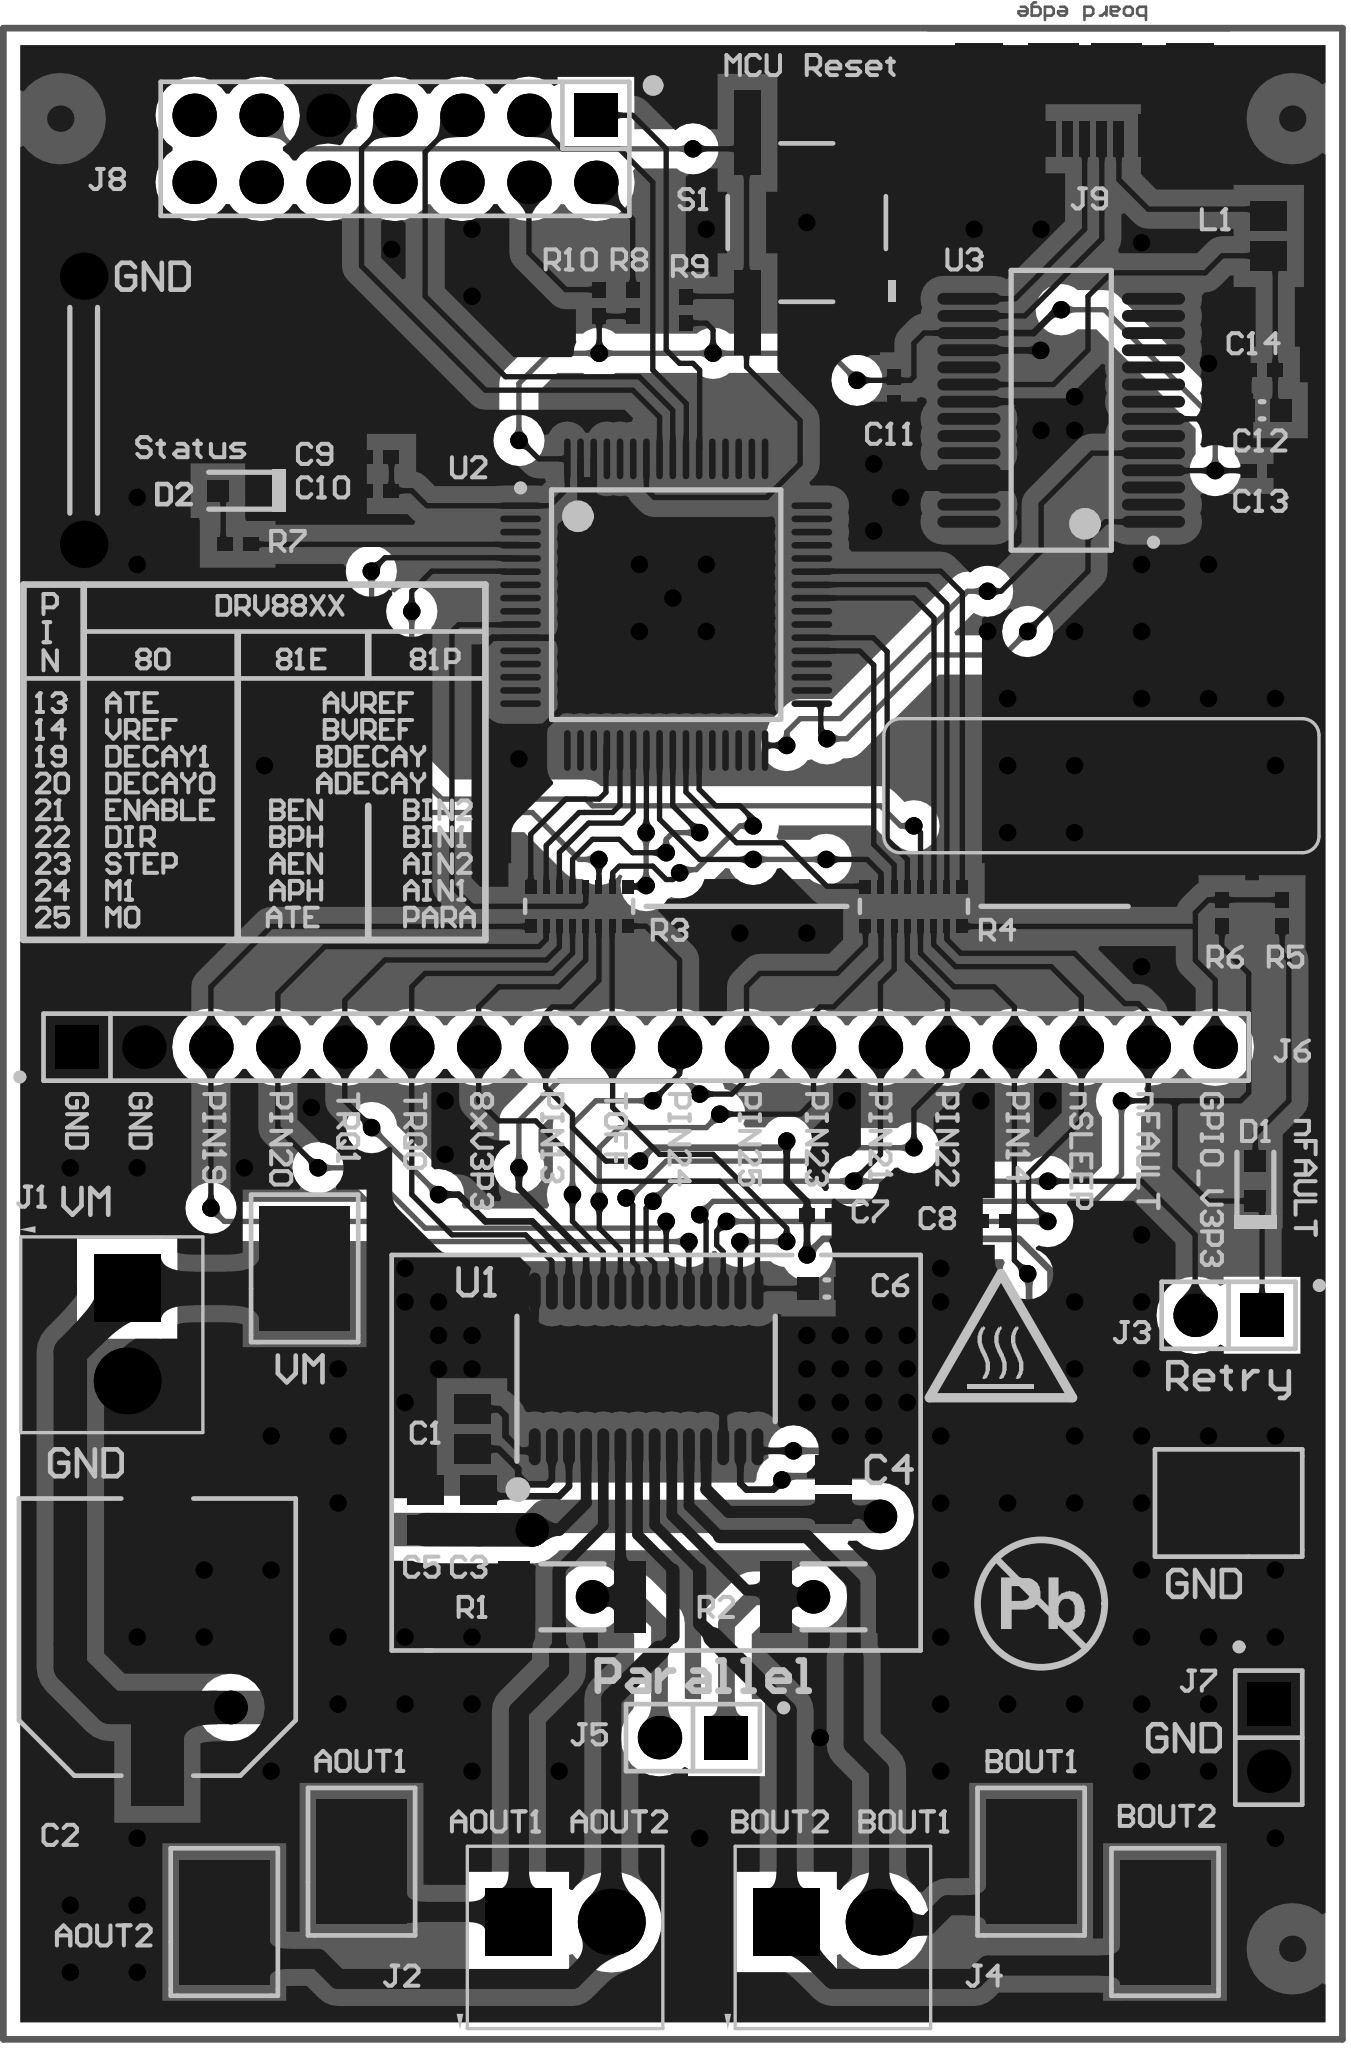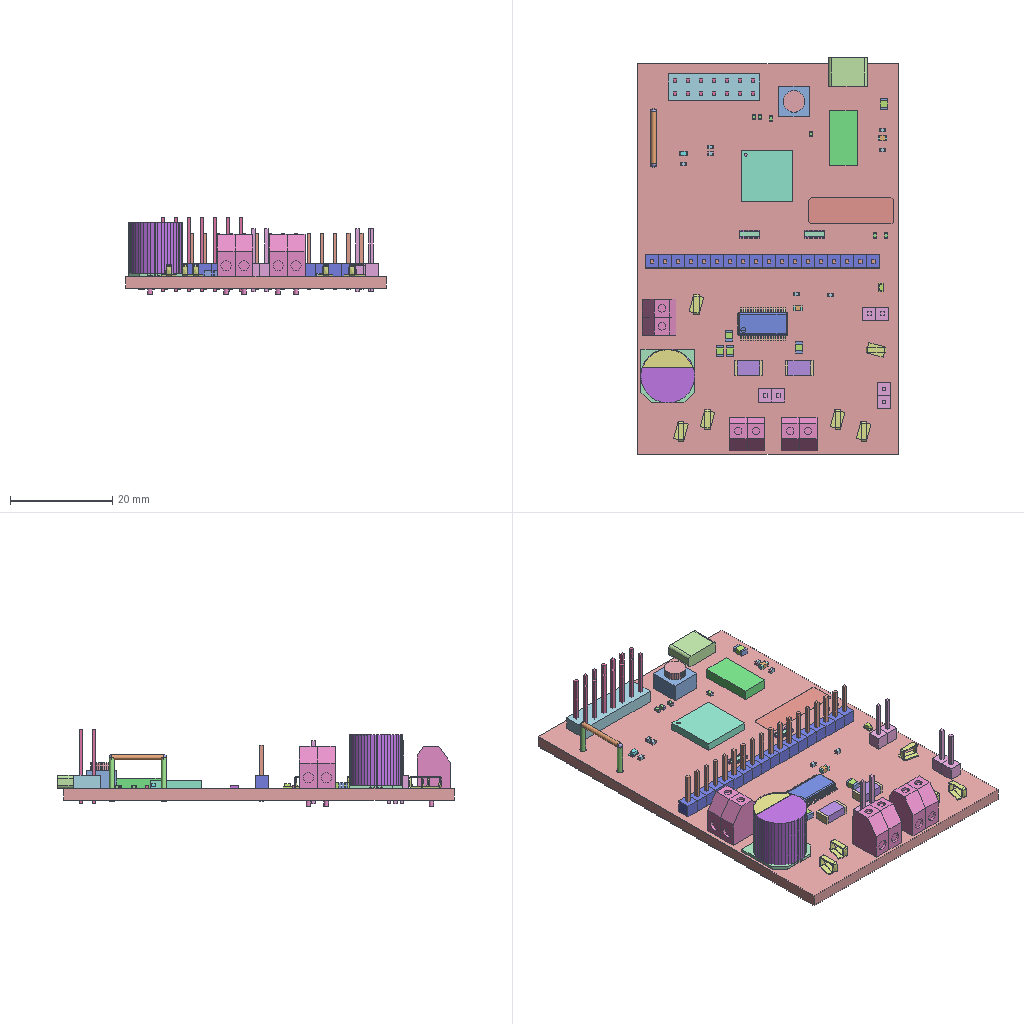Circuit board layout | Altium Designer | box 50.8 x 77.3 x 14.9 mm
Layer stack:
# Altium Designer layer stack of  (unit mm; dielectric type: 0 none, 1 core, 2 prepreg, 3 surface material)
index,name,kind,layer,copper_thickness_mm,dielectric_type,dielectric_thickness_mm,dielectric_material,dielectric_constant
0,Top Paste,other,,,,,,
1,Top Overlay,other,,,,,,
2,Top Solder,dielectric,,,3,0.0102,Solder Resist,3.5
3,Top Layer,copper,Top Layer,0.0533,,,,
4,Dielectric1,dielectric,,,1,1.504,FR-4,4.8
5,GND1,copper,GND1,0.0356,,,,
6,Dielectric2,dielectric,,,2,0.32,FR-4,4.8
7,GND2,copper,GND2,0.0356,,,,
8,Dielectric3,dielectric,,,1,0.32,FR-4,4.8
9,Bottom Layer,copper,Bottom Layer,0.0533,,,,
10,Bottom Solder,dielectric,,,3,0.0102,Solder Resist,3.5
11,Bottom Overlay,other,,,,,,
12,Bottom Paste,other,,,,,,
# drill layer pairs: low layer,high layer
drill_pair,Top Layer,Bottom Layer
Part placement:
Designator,Comment,Layer,Footprint,Center-X(mm),Center-Y(mm),Rotation
FID3,Fiducial,TopLayer,Fiducial10-20,48.895,3.429,90
FID2,Fiducial,TopLayer,Fiducial10-20,48.895,72.771,90
FID1,Fiducial,TopLayer,Fiducial10-20,2.159,72.771,90
Logo3,Pb-Free Symbol,TopLayer,Pb-Free_Overlay_Medium,-17.577,-38.964,0
C4,C0805C104K1RACTU,TopLayer,0805L,31.496,20.828,270
C5,C0805C104K1RACTU,TopLayer,0805L,16.002,20.066,270
J7,90120-0122,TopLayer,CONN_90120-0122,48.006,11.43,270
J3,90120-0122,TopLayer,CONN_90120-0122,46.482,27.432,180
J5,90120-0122,TopLayer,CONN_90120-0122,26.162,11.43,180
C12,CGB3B1X5R1A475K055AC,TopLayer,0603L,47.752,61.722,180
R10,ERJ-2GE0R00X,TopLayer,0402L,22.606,65.786,90
R8,ERJ-2GE0R00X,TopLayer,0402L,23.876,65.786,90
C14,GRM155R61A104KA01D,TopLayer,0402L,47.752,63.246,180
TP6,5016,TopLayer,Testpoint_Keystone_Compact,44.069,4.445,90
TP5,5016,TopLayer,Testpoint_Keystone_Compact,38.989,6.731,90
TP4,5016,TopLayer,Testpoint_Keystone_Compact,8.382,4.445,90
TP3,5016,TopLayer,Testpoint_Keystone_Compact,13.589,6.731,90
TP2,5016,TopLayer,Testpoint_Keystone_Compact,46.482,20.32,180
R4,EXB-2HV330JV,TopLayer,RESCAXS_EXB-2HV,34.544,42.926,360
R3,EXB-2HV330JV,TopLayer,RESCAXS_EXB-2HV,21.844,42.926,360
J6,TSW-118-07-G-S,TopLayer,TSW-118-07-G-S,24.384,37.592,360
L1,MMZ2012R300A,TopLayer,0805L,48.006,68.326,90
C11,GRM155R61A104KA01D,TopLayer,0402L,33.782,62.484,270
C13,GRM155R61A105KE15D,TopLayer,0402L,47.752,59.436,360
R9,CRCW04023K32FKED,TopLayer,0402L,25.908,65.532,270
R7,CRCW0402330RJNED,TopLayer,0402L,8.89,56.642,360
R5,CRCW0402510RJNED,TopLayer,0402L,48.514,42.672,90
J9,ZX62-B-5PA(11),TopLayer,CONN_USB_micro_ZX62-B-5PA,41.021,73.347,180
J4,ED555/2DS,TopLayer,TERM_BLK_ED555-2DS,31.471,4.445,0
J2,ED555/2DS,TopLayer,TERM_BLK_ED555-2DS,21.311,4.445,0
J1,ED555/2DS,TopLayer,TERM_BLK_ED555-2DS,4.699,26.695,270
D2,LTST-C190GKT,TopLayer,LED_LTST-C190,8.89,58.674,360
R1,CSRN2010FKR250,TopLayer,2010L,21.59,16.764,360
U3,FT232RL,TopLayer,SSOP28_M,40.132,61.722,180
S1,EVQP1D05M,TopLayer,SW_EVQxxx05M,30.48,68.834,180
D1,LTST-C190CKT,TopLayer,LED_LTST-C190_Red,47.498,32.512,270
C9,GRM155R61A104KA01D,TopLayer,0402L,14.224,59.944,180
R2,CSRN2010FKR250,TopLayer,2010L,31.496,16.764,180
U2,MSP430F2617TPM,TopLayer,PM0064A_L,25.146,54.356,0
LOGO1,CAUTION HOT SURFACE,TopLayer,IEC_HotSurface_Small,-17.577,-38.964,360
TP7,D3082-05,TopLayer,Harwin_D3082-05,3.048,61.722,270
R6,CRCW04024K99FKED,TopLayer,0402L,46.228,42.672,90
C7,GRM155R61A104KA01D,TopLayer,0402L,30.988,31.242,360
C1,C0805C104K1RACTU,TopLayer,0805L,17.78,23.114,270
C3,C2012X7R1E474K,TopLayer,0805L,18.034,20.066,270
TP1,5016,TopLayer,Testpoint_Keystone_Compact,11.43,29.21,90
J8,PEC07DAAN,TopLayer,CONN_PEC07DAAN,14.859,71.628,180
C8,GRM155R61A104KA01D,TopLayer,0402L,37.592,30.988,180
C10,GRM155R61A104KA01D,TopLayer,0402L,14.224,58.674,180
C6,C0603C474K9RACTU,TopLayer,0603L,31.242,28.448,360
C2,EEE-FK1J101P,TopLayer,SM_RADIAL_G,5.842,15.24,90
LBL1,Size: 0.65 x 0.20 "",TopLayer,Label_650x200,41.656,47.498,0,000 per roll"
U1,DRV8880PWPR,TopLayer,PWP0028C_N,24.384,25.4,90
Pad and via stacks:
# Altium Designer via and pad stacks of  (unit mm). Each distinct definition once, with the count of objects using it.
# via: kind,start_layer,end_layer,hole_mm,diameter_mm,mode(0 simple;1 top-mid-bottom;2 full stack),diameter_per_layer,count,example_net
# pad: kind,layer,hole_mm,hole_type(0 round;1 square;2 slot),plating,top_size,top_shape(1 round;2 rect;3 octagon;9 rounded rect),mid_size,bottom_size,mode,footprint,size_per_layer,count,example
pad,Top Layer,0,0,plated,0.45x2.4,1,0.45x2.4,0.45x2.4,0,SSOP28_M,,28,U3.1
pad,Top Layer,0,0,plated,0.25x1.55,1,0.25x1.55,0.25x1.55,0,PM0064A_L,,64,U2.1
pad,Top Layer,0,0,plated,3.1x5.18,9,3.1x5.18,3.1x5.18,0,PWP0028C_N,,1,U1.29
pad,Top Layer,0,0,plated,0.45x1.4,9,0.45x1.4,0.45x1.4,0,PWP0028C_N,,28,U1.15
pad,Top Layer,0,0,plated,4.699x3.429,2,4.699x3.429,4.699x3.429,0,Testpoint_Keystone_Compact,,6,TP6.1
pad,Top Layer,0,0,plated,1x3.2,2,1x3.2,1x3.2,0,SW_EVQxxx05M,,4,S1.4
pad,Top Layer,0,0,plated,0.5x0.6,2,0.5x0.6,0.5x0.6,0,0402L,,26,R10.2
pad,Top Layer,0,0,plated,0.425x0.5,2,0.425x0.5,0.425x0.5,0,RESCAXS_EXB-2HV,,8,R4.1
pad,Top Layer,0,0,plated,0.25x0.5,2,0.25x0.5,0.25x0.5,0,RESCAXS_EXB-2HV,,24,R4.2
pad,Top Layer,0,0,plated,2.7x1.2,2,2.7x1.2,2.7x1.2,0,2010L,,4,R2.2
pad,Top Layer,0,0,plated,1.4x1.1,2,1.4x1.1,1.4x1.1,0,0805L,,10,L1.2
pad,Top Layer,0,0,plated,2.1x1.6,2,2.1x1.6,2.1x1.6,0,CONN_USB_micro_ZX62-B-5PA,,2,J9.11
pad,Top Layer,0,0,plated,1.8x1.9,2,1.8x1.9,1.8x1.9,0,CONN_USB_micro_ZX62-B-5PA,,2,J9.9
pad,Top Layer,0,0,plated,1.9x1.9,2,1.9x1.9,1.9x1.9,0,CONN_USB_micro_ZX62-B-5PA,,2,J9.6
pad,Top Layer,0,0,plated,0.4x1.35,2,0.4x1.35,0.4x1.35,0,CONN_USB_micro_ZX62-B-5PA,,5,J9.1
pad,Top Layer,0,0,plated,1x1,1,1x1,1x1,0,Fiducial10-20,,3,FID3.1
pad,Top Layer,0,0,plated,0.8x0.8,2,0.8x0.8,0.8x0.8,0,LED_LTST-C190,,2,D2.1
pad,Top Layer,0,0,plated,0.8x0.8,2,0.8x0.8,0.8x0.8,0,LED_LTST-C190_Red,,2,D1.2
pad,Top Layer,0,0,plated,0.85x0.8,2,0.85x0.8,0.85x0.8,0,0603L,,4,C12.2
pad,Top Layer,0,0,plated,4.1x2,2,4.1x2,4.1x2,0,SM_RADIAL_G,,2,C2.1
pad,M13 Component Bodies Top,0,0,plated,0.0254x0.0254,1,0.0254x0.0254,0.0254x0.0254,0,Label_650x200,,1,LBL1.0
pad,Multi-Layer,1.3,0,plated,1.8x1.8,1,1.8x1.8,1.8x1.8,0,Harwin_D3082-05,,2,TP7.2
pad,Multi-Layer,1.016,0,plated,1.65x1.65,2,1.65x1.65,1.65x1.65,0,CONN_PEC07DAAN,,1,J8.1
pad,Multi-Layer,1.016,0,plated,1.65x1.65,1,1.65x1.65,1.65x1.65,0,CONN_PEC07DAAN,,13,J8.2
pad,Multi-Layer,1.016,0,plated,1.65x1.65,1,1.65x1.65,1.65x1.65,0,CONN_90120-0122,,3,J7.2
pad,Multi-Layer,1.016,0,plated,1.65x1.65,2,1.65x1.65,1.65x1.65,0,CONN_90120-0122,,3,J7.1
pad,Multi-Layer,1.016,0,plated,1.65x1.65,2,1.65x1.65,1.65x1.65,0,TSW-118-07-G-S,,1,J6.1
pad,Multi-Layer,1.016,0,plated,1.65x1.65,1,1.65x1.65,1.65x1.65,0,TSW-118-07-G-S,,17,J6.2
pad,Multi-Layer,1.27,0,plated,2.54x2.54,2,2.54x2.54,2.54x2.54,0,TERM_BLK_ED555-2DS,,3,J4.1
pad,Multi-Layer,1.27,0,plated,2.54x2.54,1,2.54x2.54,2.54x2.54,0,TERM_BLK_ED555-2DS,,3,J4.2
via,Top Layer,Bottom Layer,0.2,0.5,0,,15,GND
via,Top Layer,Bottom Layer,0.7112,1.27,0,,5,VM
via,Top Layer,Bottom Layer,0.2032,0.6604,0,,181,V3P3
Copper pours:
name,layer,net,type(0 solid;1 hatched;2 none)
Top Layer-GND,Top Layer,GND,0
Bottom Layer-GND,Bottom Layer,GND,0
Design rules, without the lines most boards share, first 41 of 43 lines:
# Altium Designer design rules of  (exported by Altium Designer, unit mm)
# columns: name | kind | enabled | priority | scope1 | scope2 | descriptor | typed fields (field=value)
PolygonConnect_2 | 20 | enabled | 1 | All | IsNamedPolygon('Top Layer-GND') | Polygon Connect Rule(Direct Connect )(Conductor Width=10mil) (Relief Angle=90 Angle) (Entries=4) (Air Gap Width=10mil) (All),(IsNamedPolygon('Top Layer-GND')) | connect_style(0=relief,1=direct,2=none)=1 relief_conductor_width=0.254 relief_entries=4
PolygonConnect_1 | 20 | enabled | 2 | All | IsNamedPolygon('Bottom Layer-GND') | Polygon Connect Rule(Direct Connect )(Conductor Width=10mil) (Relief Angle=90 Angle) (Entries=4) (Air Gap Width=10mil) (All),(IsNamedPolygon('Bottom Layer-GND')) | connect_style(0=relief,1=direct,2=none)=1 relief_conductor_width=0.254 relief_entries=4
SilkToSilkClearance | 55 | enabled | 2 | All | All | Silk to Silk (Clearance=3mil) (All),(All) |
SilkToSilkClearance_Pb-FreeLogo | 55 | enabled | 1 | (HasFootprint('Pb-Free_Overlay_Medium') OR HasFootprint('Pb-Free_Overlay_Small')) | (HasFootprint('Pb-Free_Overlay_Medium') OR HasFootprint('Pb-Free_Overlay_Small')) | Silk to Silk (Clearance=0mil) ((HasFootprint('Pb-Free_Overlay_Medium') OR HasFootprint('Pb-Free_Overlay_Small'))),((HasFootprint('Pb-Free_Overlay_Medium') OR HasFootprint('Pb-Free_Overlay_Small'))) |
Silk to Solder Mask Opening | 54 | enabled | 1 | IsPad | All | Silk To Solder Mask (Clearance=3mil) (IsPad),(All) |
MinimumSolderMaskSliver | 53 | enabled | 2 | All | All | Minimum Solder Mask Sliver (Gap=3.937mil) (All),(All) |
MinimumSolderMaskSliver_Logo | 53 | enabled | 1 | InComponentClass('Logo') | InComponentClass('Logo') | Minimum Solder Mask Sliver (Gap=0.7mil) (InComponentClass('Logo')),(InComponentClass('Logo')) |
HoleToHoleClearance | 52 | enabled | 1 | All | All | Hole To Hole Clearance (Gap=10mil) (All),(All) | gap=0.254
DiffPairsRouting | 51 | enabled | 1 | All | All | Differential Pairs Uncoupled Length using the Gap Constraints (Min=10mil) (Max=100mil) (Prefered=10mil)  and Width Constraints (Min=15mil) (Max=15mil) (Prefered=15mil) (All) |
Fanout_Small | 49 | enabled | 5 | (CompPinCount < 5) | All | Fanout Control Rule ( ((CompPinCount < 5)) ) |
Fanout_Default | 49 | enabled | 4 | All | All | Fanout Control Rule ( (All) ) |
Fanout_BGA | 49 | enabled | 2 | IsBGA | All | Fanout Control Rule ( (IsBGA) ) |
Fanout_LCC | 49 | enabled | 1 | IsLCC | All | Fanout Control Rule ( (IsLCC) ) |
TestPointUsage | 44 | enabled | 1 | All | All | Fabrication Testpoint Usage (Valid =Don't care, Allow multiple per net=No) (All) |
Testpoint | 43 | enabled | 1 | (IsPad And (OnTopLayer Or OnBottomLayer)) | All | Fabrication Testpoint Style (Under Component=Yes) ((IsPad And (OnTopLayer Or OnBottomLayer))) |
HoleSize | 42 | enabled | 1 | All | All | Hole Size Constraint (Min=7.874mil) (Max=251mil) (All) |
ComponentClearance | 24 | enabled | 9 | All | All | Component Clearance Constraint ( Horizontal Gap = 40mil, Vertical Gap = 10mil ) (All),(All)  | gap=1.016
ComponentClearance_THtoTH | 24 | enabled | 8 | IsThruComponent | IsThruComponent | Component Clearance Constraint ( Horizontal Gap = 118.11mil, Vertical Gap = 30mil ) (IsThruComponent),(IsThruComponent)  | gap=3
ComponentClearance_THtoSMT | 24 | enabled | 7 | IsThruComponent | IsSMTComponent | Component Clearance Constraint ( Horizontal Gap = 100mil, Vertical Gap = 30mil ) (IsThruComponent),(IsSMTComponent)  | gap=2.54
ComponentClearance_SmallPassives | 24 | enabled | 6 | HasFootprint('0201*') or HasFootprint('0402*') or HasFootprint('0508') or HasFootprint('0603*') or HasFootprint('0612') or HasFootprint('0805*') or HasFootprint('0815*') or HasFootprint('0830*') or HasFootprint('1206*') or HasFootprint('1210*') or HasFootprint('1808*') or HasFootprint('1812*') or HasFootprint('1825*') or HasFootprint('2010*') or HasFootprint('2220*') or HasFootprint('2225*') or HasFootprint('2512*') or HasFootprint('2728*') or HasFootprint('3518*') | HasFootprint('0201*') or HasFootprint('0402*') or HasFootprint('0508') or HasFootprint('0603*') or HasFootprint('0612') or HasFootprint('0805*') or HasFootprint('0815*') or HasFootprint('0830*') or HasFootprint('1206*') or HasFootprint('1210*') or HasFootprint('1808*') or HasFootprint('1812*') or HasFootprint('1825*') or HasFootprint('2010*') or HasFootprint('2220*') or HasFootprint('2225*') or HasFootprint('2512*') or HasFootprint('2728*') or HasFootprint('3518*') | Component Clearance Constraint ( Horizontal Gap = 20mil, Vertical Gap = 10mil ) (HasFootprint('0201*') or HasFootprint('0402*') or HasFootprint('0508') or HasFootprint('0603*') or HasFootprint('0612') or HasFootprint('0805*') or HasFootprint('0815*') or HasFootprint('0830*') or HasFootprint('1206*') or HasFootprint('1210*') or HasFootprint('1808*') or HasFootprint('1812*') or HasFootprint('1825*') or HasFootprint('2010*') or HasFootprint('2220*') or HasFootprint('2225*') or HasFootprint('2512*') or HasFootprint('2728*') or HasFootprint('3518*')),(HasFootprint('0201*') or HasFootprint('0402*') or HasFootprint('0508') or HasFootprint('0603*') or HasFootprint('0612') or HasFootprint('0805*') or HasFootprint('0815*') or HasFootprint('0830*') or HasFootprint('1206*') or HasFootprint('1210*') or HasFootprint('1808*') or HasFootprint('1812*') or HasFootprint('1825*') or HasFootprint('2010*') or HasFootprint('2220*') or HasFootprint('2225*') or HasFootprint('2512*') or HasFootprint('2728*') or HasFootprint('3518*'))  | gap=0.508
ComponentClearance_MountingHoles | 24 | enabled | 5 | InComponentClass('Mounting Holes') | All | Component Clearance Constraint ( Horizontal Gap = 250mil, Vertical Gap = Infinite ) (InComponentClass('Mounting Holes')),(All)  | gap=6.35
ComponentClearance_ScrewToNut | 24 | enabled | 4 | (HasFootprint('NY PMS 440 0025 PH')) | (HasFootprint('Keystone_1902C')) | Component Clearance Constraint ( Horizontal Gap = 5mil, Vertical Gap = 10mil ) ((HasFootprint('NY PMS 440 0025 PH'))),((HasFootprint('Keystone_1902C')))  | gap=0.127
ComponentClearance_Logo | 24 | enabled | 3 | InComponentClass('Logo') | All | Component Clearance Constraint ( Horizontal Gap = 50mil, Vertical Gap = 10mil ) (InComponentClass('Logo')),(All)  | gap=1.27
ComponentClearance_Shunt | 24 | enabled | 2 | InComponentClass('Header') | InComponentClass('Shunt') | Component Clearance Constraint ( Horizontal Gap = 0mil, Vertical Gap = 0mil ) (InComponentClass('Header')),(InComponentClass('Shunt'))  | gap=0
ComponentClearance_MountingHoles_FiducialMarks | 24 | enabled | 1 | InComponentClass('Mounting Holes') | InComponentClass('FiducialMark') | Component Clearance Constraint ( Horizontal Gap = 50mil, Vertical Gap = 10mil ) (InComponentClass('Mounting Holes')),(InComponentClass('FiducialMark'))  | gap=1.27
AcuteAngle | 21 | enabled | 1 | All | All | Acute Angle Constraint (Minimum=45.000) (All) |
PolygonConnect | 20 | enabled | 3 | All | All | Polygon Connect Rule(Relief Connect )(Conductor Width=10mil) (Relief Angle=90 Angle) (Entries=4) (Air Gap Width=10mil) (All),(All) | connect_style(0=relief,1=direct,2=none)=0 relief_conductor_width=0.254 relief_entries=4
MinimumAnnularRing | 19 | enabled | 2 | All | All | Minimum Annular Ring (Minimum=5mil) (All) |
MinimumAnnularRing_ThermalPadVias | 19 | enabled | 1 | IsVia and InAnyComponent | All | Minimum Annular Ring (Minimum=3.937mil) (IsVia and InAnyComponent) |
PasteMaskExpansion | 14 | enabled | 1 | All | All | Paste Mask Expansion (Expansion =0mil) (All) | expansion=0
SolderMaskExpansion | 13 | enabled | 1 | All | All | Solder Mask Expansion (Expansion =1.968mil) (All) | expansion=0.05
RoutingVias | 11 | enabled | 2 | All | All | Routing Via (MinHoleWidth=7.874mil) (MaxHoleWidth=40mil) (PreferredHoleWidth=16mil) (MinWidth=26mil) (MaxWidth=65mil) (PreferedWidth=34mil) (All) | via_min_hole=0.2 via_max_hole=1.016 via_preferred_diameter=0.8636 via_preferred_hole=0.4064
ThermalPadVias | 11 | enabled | 1 | IsVia and InAnyComponent | All | Routing Via (MinHoleWidth=7.874mil) (MaxHoleWidth=12.992mil) (PreferredHoleWidth=7.874mil) (MinWidth=15.748mil) (MaxWidth=23.622mil) (PreferedWidth=19.685mil) (IsVia and InAnyComponent) | via_min_hole=0.2 via_max_hole=0.33 via_preferred_diameter=0.5 via_preferred_hole=0.2
PlaneConnect | 6 | enabled | 1 | All | All | Power Plane Connect Rule(Relief Connect )(Expansion=10mil) (Conductor Width=10mil) (Air Gap=10mil) (Entries=4) (All) | relief_conductor_width=0.254 relief_entries=4 relief_expansion=0.254
Width | 2 | enabled | 1 | All | All | Width Constraint (Min=6mil) (Max=100mil) (Preferred=10mil) (All) |
Clearance | 0 | enabled | 6 | All | All | Clearance Constraint (Gap=7.874mil) (All),(All) | gap=0.2
Clearance_Poly | 0 | enabled | 5 | InPolygon | All | Clearance Constraint (Gap=25mil) (InPolygon),(All) | gap=0.635
Clearance_BoardEdge | 0 | enabled | 4 | OnCopper and Not InComponentClass('Logo') and not InComponentClass('FiducialMark') and not InRegion(1000,500,4000,800) and Not IsKeepout | IsKeepOut | Clearance Constraint (Gap=20mil) (OnCopper and Not InComponentClass('Logo') and not InComponentClass('FiducialMark') and not InRegion(1000,500,4000,800) and Not IsKeepout),(IsKeepOut) | gap=0.508
Clearance_BoardEdge_Poly | 0 | enabled | 3 | OnCopper and InPoly | IsKeepOut | Clearance Constraint (Gap=25mil) (OnCopper and InPoly),(IsKeepOut) | gap=0.635
Classes set for this board:
# Altium Designer classes of  (member kind: 0 net, 1 component, 2 from-to, 3 pad, 4 layer, 5 differential pair, 6 design channel, 7 polygon, 8 structure, 9 xSignal)
# columns: class name | member kind | superclass | members
Header | 1 | no | J6; J3; J5; J7; J8;
MDBU004A_DRV888x | 1 | no | C1; C2; C3; C4; C5; C6; C7; C8; D1; J1; J2; J3; J4; J5; J6; J7; R1; R2; R3; R4; R5; R6; U1; TP4; TP3; TP1; TP6; TP2; TP5; TP7;
MDBU004A_DRV888x_MSP430F2617 | 1 | no | C9; C10; C11; C12; C13; C14; D2; J8; J9; L1; R7; R8; R9; R10; S1; U2; U3;
Logo | 1 | no | Logo2;
MDBU004A_Hardware | 1 | no | FID1; FID2; FID3; LBL1; LOGO1; Logo2; Logo3; Logo4; ZZ1; ZZ2; ZZ3; ZZ4; ZZ5;
FiducialMark | 1 | no | FID1; FID2; FID3;
AssemblyNote | 1 | no | ZZ1; ZZ2; ZZ3; ZZ4; ZZ5;
Label | 1 | no | LBL1;